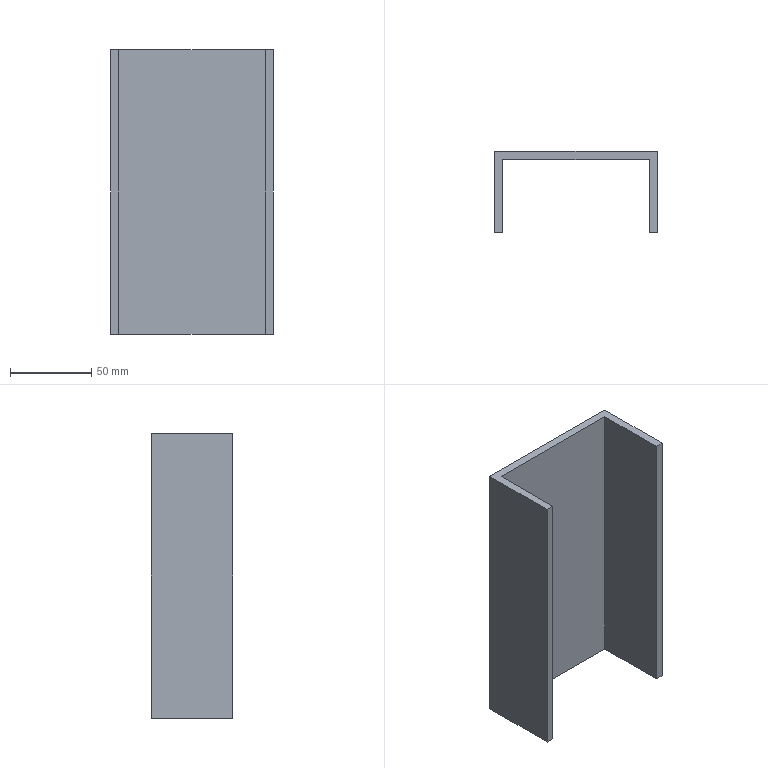Part | SolidWorks | features Extrusion 1 | 1 solid | 10 faces | box 100 x 50 x 175 mm | volume 166250 mm3 | plane 10
STEP:
#1=CARTESIAN_POINT('',(0.,0.,0.));
#2=VERTEX_POINT('',#1);
#3=CARTESIAN_POINT('',(0.,-50.,0.));
#4=VERTEX_POINT('',#3);
#5=CARTESIAN_POINT('',(0.,0.,0.));
#6=DIRECTION('',(0.,-1.,0.));
#7=VECTOR('',#6,1000.);
#8=LINE('',#5,#7);
#9=EDGE_CURVE('',#2,#4,#8,.T.);
#10=ORIENTED_EDGE('',*,*,#9,.T.);
#11=CARTESIAN_POINT('',(0.,-50.,175.));
#12=VERTEX_POINT('',#11);
#13=CARTESIAN_POINT('',(0.,-50.,175.));
#14=DIRECTION('',(0.,0.,-1.));
#15=VECTOR('',#14,1000.);
#16=LINE('',#13,#15);
#17=EDGE_CURVE('',#12,#4,#16,.T.);
#18=ORIENTED_EDGE('',*,*,#17,.F.);
#19=CARTESIAN_POINT('',(0.,0.,175.));
#20=VERTEX_POINT('',#19);
#21=CARTESIAN_POINT('',(0.,0.,175.));
#22=DIRECTION('',(0.,-1.,0.));
#23=VECTOR('',#22,1000.);
#24=LINE('',#21,#23);
#25=EDGE_CURVE('',#20,#12,#24,.T.);
#26=ORIENTED_EDGE('',*,*,#25,.F.);
#27=CARTESIAN_POINT('',(0.,0.,175.));
#28=DIRECTION('',(0.,0.,-1.));
#29=VECTOR('',#28,1000.);
#30=LINE('',#27,#29);
#31=EDGE_CURVE('',#20,#2,#30,.T.);
#32=ORIENTED_EDGE('',*,*,#31,.T.);
#33=EDGE_LOOP('',(#10,#18,#26,#32));
#34=FACE_OUTER_BOUND('',#33,.T.);
#35=CARTESIAN_POINT('',(0.,0.,175.));
#36=DIRECTION('',(1.,0.,0.));
#37=DIRECTION('',(0.,0.,-1.));
#38=AXIS2_PLACEMENT_3D('',#35,#36,#37);
#39=PLANE('',#38);
#40=ADVANCED_FACE('',(#34),#39,.F.);
#41=CARTESIAN_POINT('',(5.,-50.,0.));
#42=VERTEX_POINT('',#41);
#43=CARTESIAN_POINT('',(0.,-50.,0.));
#44=DIRECTION('',(1.,0.,0.));
#45=VECTOR('',#44,1000.);
#46=LINE('',#43,#45);
#47=EDGE_CURVE('',#4,#42,#46,.T.);
#48=ORIENTED_EDGE('',*,*,#47,.T.);
#49=CARTESIAN_POINT('',(5.,-50.,175.));
#50=VERTEX_POINT('',#49);
#51=CARTESIAN_POINT('',(5.,-50.,175.));
#52=DIRECTION('',(0.,0.,-1.));
#53=VECTOR('',#52,1000.);
#54=LINE('',#51,#53);
#55=EDGE_CURVE('',#50,#42,#54,.T.);
#56=ORIENTED_EDGE('',*,*,#55,.F.);
#57=CARTESIAN_POINT('',(0.,-50.,175.));
#58=DIRECTION('',(1.,0.,0.));
#59=VECTOR('',#58,1000.);
#60=LINE('',#57,#59);
#61=EDGE_CURVE('',#12,#50,#60,.T.);
#62=ORIENTED_EDGE('',*,*,#61,.F.);
#63=ORIENTED_EDGE('',*,*,#17,.T.);
#64=EDGE_LOOP('',(#48,#56,#62,#63));
#65=FACE_OUTER_BOUND('',#64,.T.);
#66=CARTESIAN_POINT('',(0.,-50.,175.));
#67=DIRECTION('',(0.,1.,0.));
#68=DIRECTION('',(0.,0.,1.));
#69=AXIS2_PLACEMENT_3D('',#66,#67,#68);
#70=PLANE('',#69);
#71=ADVANCED_FACE('',(#65),#70,.F.);
#72=CARTESIAN_POINT('',(5.,-5.,0.));
#73=VERTEX_POINT('',#72);
#74=CARTESIAN_POINT('',(5.,-5.,0.));
#75=DIRECTION('',(0.,1.,0.));
#76=VECTOR('',#75,1000.);
#77=LINE('',#74,#76);
#78=EDGE_CURVE('',#42,#73,#77,.T.);
#79=ORIENTED_EDGE('',*,*,#78,.T.);
#80=CARTESIAN_POINT('',(5.,-5.,175.));
#81=VERTEX_POINT('',#80);
#82=CARTESIAN_POINT('',(5.,-5.,175.));
#83=DIRECTION('',(0.,0.,-1.));
#84=VECTOR('',#83,1000.);
#85=LINE('',#82,#84);
#86=EDGE_CURVE('',#81,#73,#85,.T.);
#87=ORIENTED_EDGE('',*,*,#86,.F.);
#88=CARTESIAN_POINT('',(5.,-5.,175.));
#89=DIRECTION('',(0.,1.,0.));
#90=VECTOR('',#89,1000.);
#91=LINE('',#88,#90);
#92=EDGE_CURVE('',#50,#81,#91,.T.);
#93=ORIENTED_EDGE('',*,*,#92,.F.);
#94=ORIENTED_EDGE('',*,*,#55,.T.);
#95=EDGE_LOOP('',(#79,#87,#93,#94));
#96=FACE_OUTER_BOUND('',#95,.T.);
#97=CARTESIAN_POINT('',(5.,-5.,175.));
#98=DIRECTION('',(-1.,0.,0.));
#99=DIRECTION('',(0.,0.,1.));
#100=AXIS2_PLACEMENT_3D('',#97,#98,#99);
#101=PLANE('',#100);
#102=ADVANCED_FACE('',(#96),#101,.F.);
#103=CARTESIAN_POINT('',(95.,-5.,0.));
#104=VERTEX_POINT('',#103);
#105=CARTESIAN_POINT('',(5.,-5.,0.));
#106=DIRECTION('',(1.,0.,0.));
#107=VECTOR('',#106,1000.);
#108=LINE('',#105,#107);
#109=EDGE_CURVE('',#73,#104,#108,.T.);
#110=ORIENTED_EDGE('',*,*,#109,.T.);
#111=CARTESIAN_POINT('',(95.,-5.,175.));
#112=VERTEX_POINT('',#111);
#113=CARTESIAN_POINT('',(95.,-5.,175.));
#114=DIRECTION('',(0.,0.,-1.));
#115=VECTOR('',#114,1000.);
#116=LINE('',#113,#115);
#117=EDGE_CURVE('',#112,#104,#116,.T.);
#118=ORIENTED_EDGE('',*,*,#117,.F.);
#119=CARTESIAN_POINT('',(5.,-5.,175.));
#120=DIRECTION('',(1.,0.,0.));
#121=VECTOR('',#120,1000.);
#122=LINE('',#119,#121);
#123=EDGE_CURVE('',#81,#112,#122,.T.);
#124=ORIENTED_EDGE('',*,*,#123,.F.);
#125=ORIENTED_EDGE('',*,*,#86,.T.);
#126=EDGE_LOOP('',(#110,#118,#124,#125));
#127=FACE_OUTER_BOUND('',#126,.T.);
#128=CARTESIAN_POINT('',(5.,-5.,175.));
#129=DIRECTION('',(0.,1.,0.));
#130=DIRECTION('',(0.,0.,1.));
#131=AXIS2_PLACEMENT_3D('',#128,#129,#130);
#132=PLANE('',#131);
#133=ADVANCED_FACE('',(#127),#132,.F.);
#134=CARTESIAN_POINT('',(95.,-50.,0.));
#135=VERTEX_POINT('',#134);
#136=CARTESIAN_POINT('',(95.,-5.,0.));
#137=DIRECTION('',(0.,-1.,0.));
#138=VECTOR('',#137,1000.);
#139=LINE('',#136,#138);
#140=EDGE_CURVE('',#104,#135,#139,.T.);
#141=ORIENTED_EDGE('',*,*,#140,.T.);
#142=CARTESIAN_POINT('',(95.,-50.,175.));
#143=VERTEX_POINT('',#142);
#144=CARTESIAN_POINT('',(95.,-50.,175.));
#145=DIRECTION('',(0.,0.,-1.));
#146=VECTOR('',#145,1000.);
#147=LINE('',#144,#146);
#148=EDGE_CURVE('',#143,#135,#147,.T.);
#149=ORIENTED_EDGE('',*,*,#148,.F.);
#150=CARTESIAN_POINT('',(95.,-5.,175.));
#151=DIRECTION('',(0.,-1.,0.));
#152=VECTOR('',#151,1000.);
#153=LINE('',#150,#152);
#154=EDGE_CURVE('',#112,#143,#153,.T.);
#155=ORIENTED_EDGE('',*,*,#154,.F.);
#156=ORIENTED_EDGE('',*,*,#117,.T.);
#157=EDGE_LOOP('',(#141,#149,#155,#156));
#158=FACE_OUTER_BOUND('',#157,.T.);
#159=CARTESIAN_POINT('',(95.,-5.,175.));
#160=DIRECTION('',(1.,0.,0.));
#161=DIRECTION('',(0.,0.,-1.));
#162=AXIS2_PLACEMENT_3D('',#159,#160,#161);
#163=PLANE('',#162);
#164=ADVANCED_FACE('',(#158),#163,.F.);
#165=CARTESIAN_POINT('',(100.,-50.,0.));
#166=VERTEX_POINT('',#165);
#167=CARTESIAN_POINT('',(95.,-50.,0.));
#168=DIRECTION('',(1.,0.,0.));
#169=VECTOR('',#168,1000.);
#170=LINE('',#167,#169);
#171=EDGE_CURVE('',#135,#166,#170,.T.);
#172=ORIENTED_EDGE('',*,*,#171,.T.);
#173=CARTESIAN_POINT('',(100.,-50.,175.));
#174=VERTEX_POINT('',#173);
#175=CARTESIAN_POINT('',(100.,-50.,175.));
#176=DIRECTION('',(0.,0.,-1.));
#177=VECTOR('',#176,1000.);
#178=LINE('',#175,#177);
#179=EDGE_CURVE('',#174,#166,#178,.T.);
#180=ORIENTED_EDGE('',*,*,#179,.F.);
#181=CARTESIAN_POINT('',(95.,-50.,175.));
#182=DIRECTION('',(1.,0.,0.));
#183=VECTOR('',#182,1000.);
#184=LINE('',#181,#183);
#185=EDGE_CURVE('',#143,#174,#184,.T.);
#186=ORIENTED_EDGE('',*,*,#185,.F.);
#187=ORIENTED_EDGE('',*,*,#148,.T.);
#188=EDGE_LOOP('',(#172,#180,#186,#187));
#189=FACE_OUTER_BOUND('',#188,.T.);
#190=CARTESIAN_POINT('',(95.,-50.,175.));
#191=DIRECTION('',(0.,1.,0.));
#192=DIRECTION('',(0.,0.,1.));
#193=AXIS2_PLACEMENT_3D('',#190,#191,#192);
#194=PLANE('',#193);
#195=ADVANCED_FACE('',(#189),#194,.F.);
#196=CARTESIAN_POINT('',(100.,0.,0.));
#197=VERTEX_POINT('',#196);
#198=CARTESIAN_POINT('',(100.,0.,0.));
#199=DIRECTION('',(0.,1.,0.));
#200=VECTOR('',#199,1000.);
#201=LINE('',#198,#200);
#202=EDGE_CURVE('',#166,#197,#201,.T.);
#203=ORIENTED_EDGE('',*,*,#202,.T.);
#204=CARTESIAN_POINT('',(100.,0.,175.));
#205=VERTEX_POINT('',#204);
#206=CARTESIAN_POINT('',(100.,0.,175.));
#207=DIRECTION('',(0.,0.,-1.));
#208=VECTOR('',#207,1000.);
#209=LINE('',#206,#208);
#210=EDGE_CURVE('',#205,#197,#209,.T.);
#211=ORIENTED_EDGE('',*,*,#210,.F.);
#212=CARTESIAN_POINT('',(100.,0.,175.));
#213=DIRECTION('',(0.,1.,0.));
#214=VECTOR('',#213,1000.);
#215=LINE('',#212,#214);
#216=EDGE_CURVE('',#174,#205,#215,.T.);
#217=ORIENTED_EDGE('',*,*,#216,.F.);
#218=ORIENTED_EDGE('',*,*,#179,.T.);
#219=EDGE_LOOP('',(#203,#211,#217,#218));
#220=FACE_OUTER_BOUND('',#219,.T.);
#221=CARTESIAN_POINT('',(100.,0.,175.));
#222=DIRECTION('',(-1.,0.,0.));
#223=DIRECTION('',(0.,0.,1.));
#224=AXIS2_PLACEMENT_3D('',#221,#222,#223);
#225=PLANE('',#224);
#226=ADVANCED_FACE('',(#220),#225,.F.);
#227=CARTESIAN_POINT('',(0.,0.,0.));
#228=DIRECTION('',(-1.,0.,0.));
#229=VECTOR('',#228,1000.);
#230=LINE('',#227,#229);
#231=EDGE_CURVE('',#197,#2,#230,.T.);
#232=ORIENTED_EDGE('',*,*,#231,.T.);
#233=ORIENTED_EDGE('',*,*,#31,.F.);
#234=CARTESIAN_POINT('',(0.,0.,175.));
#235=DIRECTION('',(-1.,0.,0.));
#236=VECTOR('',#235,1000.);
#237=LINE('',#234,#236);
#238=EDGE_CURVE('',#205,#20,#237,.T.);
#239=ORIENTED_EDGE('',*,*,#238,.F.);
#240=ORIENTED_EDGE('',*,*,#210,.T.);
#241=EDGE_LOOP('',(#232,#233,#239,#240));
#242=FACE_OUTER_BOUND('',#241,.T.);
#243=CARTESIAN_POINT('',(0.,0.,175.));
#244=DIRECTION('',(0.,-1.,0.));
#245=DIRECTION('',(0.,0.,-1.));
#246=AXIS2_PLACEMENT_3D('',#243,#244,#245);
#247=PLANE('',#246);
#248=ADVANCED_FACE('',(#242),#247,.F.);
#249=ORIENTED_EDGE('',*,*,#25,.T.);
#250=ORIENTED_EDGE('',*,*,#61,.T.);
#251=ORIENTED_EDGE('',*,*,#92,.T.);
#252=ORIENTED_EDGE('',*,*,#123,.T.);
#253=ORIENTED_EDGE('',*,*,#154,.T.);
#254=ORIENTED_EDGE('',*,*,#185,.T.);
#255=ORIENTED_EDGE('',*,*,#216,.T.);
#256=ORIENTED_EDGE('',*,*,#238,.T.);
#257=EDGE_LOOP('',(#249,#250,#251,#252,#253,#254,#255,#256));
#258=FACE_OUTER_BOUND('',#257,.T.);
#259=CARTESIAN_POINT('',(0.,0.,175.));
#260=DIRECTION('',(0.,0.,1.));
#261=DIRECTION('',(1.,0.,0.));
#262=AXIS2_PLACEMENT_3D('',#259,#260,#261);
#263=PLANE('',#262);
#264=ADVANCED_FACE('',(#258),#263,.T.);
#265=ORIENTED_EDGE('',*,*,#9,.F.);
#266=ORIENTED_EDGE('',*,*,#231,.F.);
#267=ORIENTED_EDGE('',*,*,#202,.F.);
#268=ORIENTED_EDGE('',*,*,#171,.F.);
#269=ORIENTED_EDGE('',*,*,#140,.F.);
#270=ORIENTED_EDGE('',*,*,#109,.F.);
#271=ORIENTED_EDGE('',*,*,#78,.F.);
#272=ORIENTED_EDGE('',*,*,#47,.F.);
#273=EDGE_LOOP('',(#265,#266,#267,#268,#269,#270,#271,#272));
#274=FACE_OUTER_BOUND('',#273,.T.);
#275=CARTESIAN_POINT('',(0.,0.,0.));
#276=DIRECTION('',(0.,0.,1.));
#277=DIRECTION('',(1.,0.,0.));
#278=AXIS2_PLACEMENT_3D('',#275,#276,#277);
#279=PLANE('',#278);
#280=ADVANCED_FACE('',(#274),#279,.F.);
#281=CLOSED_SHELL('',(#40,#71,#102,#133,#164,#195,#226,#248,#264,#280));
#282=MANIFOLD_SOLID_BREP('',#281);
#283=CARTESIAN_POINT('',(0.,0.,0.));
#284=DIRECTION('',(0.,0.,1.));
#285=DIRECTION('',(1.,0.,0.));
#286=AXIS2_PLACEMENT_3D('',#283,#284,#285);
#287=(LENGTH_UNIT()NAMED_UNIT(*)SI_UNIT(.MILLI.,.METRE.));
#288=UNCERTAINTY_MEASURE_WITH_UNIT(LENGTH_MEASURE(0.00001),#287,'','');
#289=(NAMED_UNIT(*)PLANE_ANGLE_UNIT()SI_UNIT($,.RADIAN.));
#290=(NAMED_UNIT(*)SI_UNIT($,.STERADIAN.)SOLID_ANGLE_UNIT());
#291=(GEOMETRIC_REPRESENTATION_CONTEXT(3)GLOBAL_UNCERTAINTY_ASSIGNED_CONTEXT((#288))GLOBAL_UNIT_ASSIGNED_CONTEXT((#287,#289,#290))REPRESENTATION_CONTEXT('',''));
#292=ADVANCED_BREP_SHAPE_REPRESENTATION('',(#282,#286),#291);